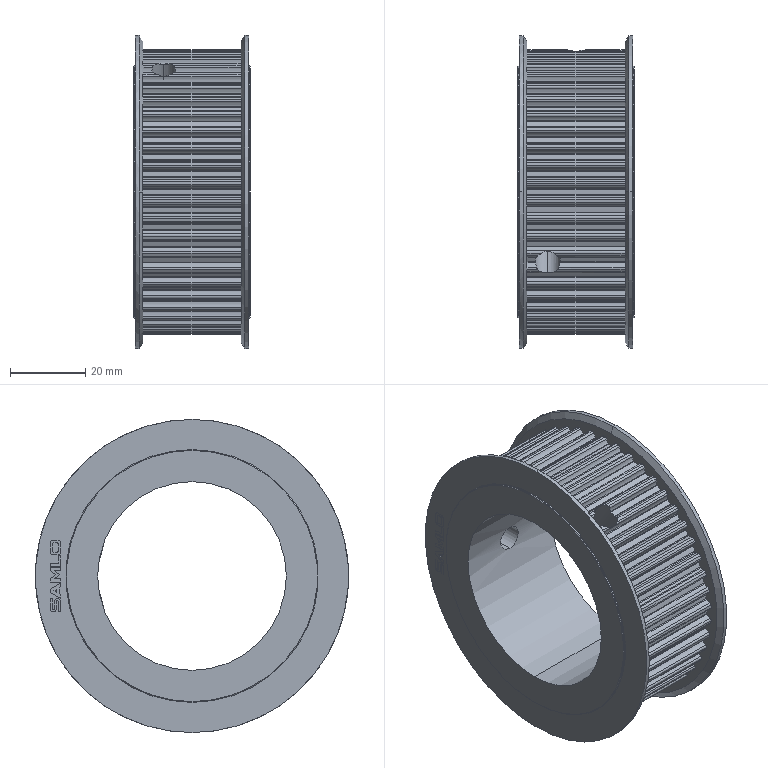Part | SolidWorks | features MoveFace 2, BaseBody 1, ICE 1 | 1 solid | 542 faces | box 31 x 83 x 83 mm | volume 73230 mm3 | cylinder 476 | plane 58 | cone 8 | commonest cylinder face diameters 1.1 x122 0.5 x115 6.55 x108 75.43 x52 71.89 x51 0.643 x4